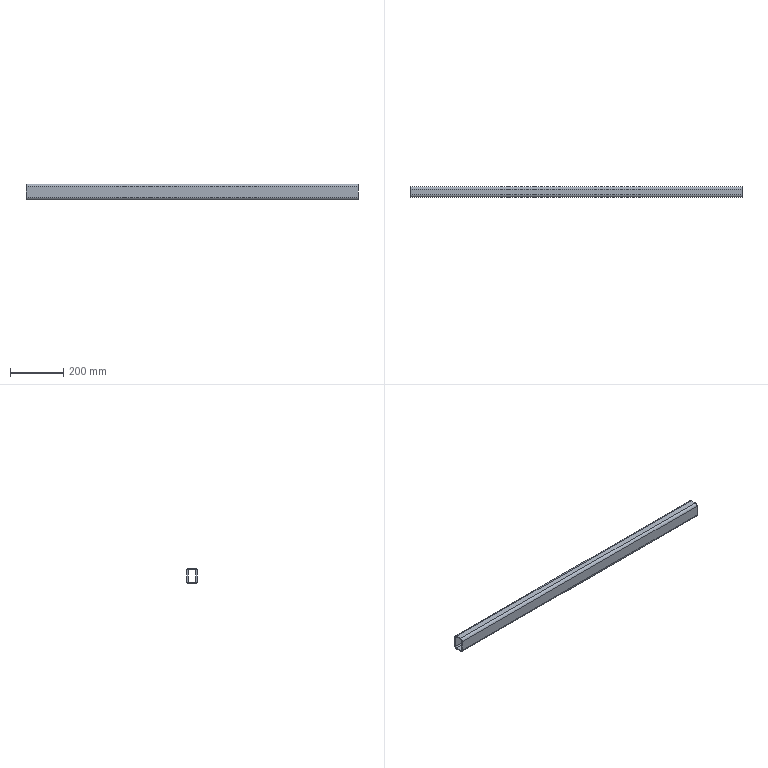Part | STEP file | HL4GD-1.30.108 base frame outer longitudinal beam--20251212 | 1 solid | 18 faces | box 1250 x 40 x 60 mm | volume 1044524 mm3 | plane 10 | cylinder 8 | commonest cylinder face diameters 10 x4 20 x4
STEP:
#1=CARTESIAN_POINT('',(0.,0.,0.));
#2=DIRECTION('',(0.,0.,1.));
#3=DIRECTION('',(1.,0.,0.));
#4=AXIS2_PLACEMENT_3D('',#1,#2,#3);
#5=CARTESIAN_POINT('',(1515.,1140.,410.));
#6=VERTEX_POINT('',#5);
#7=CARTESIAN_POINT('',(1515.,1145.,415.));
#8=VERTEX_POINT('',#7);
#9=CARTESIAN_POINT('',(1515.,1140.,415.));
#10=DIRECTION('',(1.,0.,0.));
#11=DIRECTION('',(0.,1.,0.));
#12=AXIS2_PLACEMENT_3D('',#9,#10,#11);
#13=CIRCLE('',#12,5.);
#14=CARTESIAN_POINT('',(2495.,1140.,415.));
#15=DIRECTION('',(1.,0.,0.));
#16=DIRECTION('',(0.,1.,0.));
#17=AXIS2_PLACEMENT_3D('',#14,#15,#16);
#18=CYLINDRICAL_SURFACE('',#17,5.);
#19=CARTESIAN_POINT('',(0.,-980.));
#20=DIRECTION('',(1.,0.));
#21=VECTOR('',#20,1.);
#22=LINE('',#19,#21);
#23=(GEOMETRIC_REPRESENTATION_CONTEXT(2)PARAMETRIC_REPRESENTATION_CONTEXT()REPRESENTATION_CONTEXT('',''));
#24=DEFINITIONAL_REPRESENTATION('',(#22),#23);
#25=PCURVE('',#18,#24);
#26=CARTESIAN_POINT('',(1515.,1326.07,281.07));
#27=DIRECTION('',(1.,0.,0.));
#28=DIRECTION('',(0.,1.,0.));
#29=AXIS2_PLACEMENT_3D('',#26,#27,#28);
#30=PLANE('',#29);
#31=CARTESIAN_POINT('',(-186.07,133.93));
#32=DIRECTION('',(1.,0.));
#33=AXIS2_PLACEMENT_2D('',#31,#32);
#34=CIRCLE('',#33,5.);
#35=(GEOMETRIC_REPRESENTATION_CONTEXT(2)PARAMETRIC_REPRESENTATION_CONTEXT()REPRESENTATION_CONTEXT('',''));
#36=DEFINITIONAL_REPRESENTATION('',(#34),#35);
#37=PCURVE('',#30,#36);
#38=SURFACE_CURVE('',#13,(#25,#37),.PCURVE_S1.);
#39=EDGE_CURVE('',#6,#8,#38,.T.);
#40=ORIENTED_EDGE('',*,*,#39,.T.);
#41=CARTESIAN_POINT('',(2765.,1145.,415.));
#42=VERTEX_POINT('',#41);
#43=CARTESIAN_POINT('',(2495.,1145.,415.));
#44=DIRECTION('',(1.,0.,0.));
#45=VECTOR('',#44,1.);
#46=LINE('',#43,#45);
#47=CARTESIAN_POINT('',(6.283,0.));
#48=DIRECTION('',(0.,1.));
#49=VECTOR('',#48,1.);
#50=LINE('',#47,#49);
#51=(GEOMETRIC_REPRESENTATION_CONTEXT(2)PARAMETRIC_REPRESENTATION_CONTEXT()REPRESENTATION_CONTEXT('',''));
#52=DEFINITIONAL_REPRESENTATION('',(#50),#51);
#53=PCURVE('',#18,#52);
#54=CARTESIAN_POINT('',(2495.,1145.,415.));
#55=DIRECTION('',(0.,-1.,0.));
#56=DIRECTION('',(0.,0.,-1.));
#57=AXIS2_PLACEMENT_3D('',#54,#55,#56);
#58=PLANE('',#57);
#59=CARTESIAN_POINT('',(0.,0.));
#60=DIRECTION('',(0.,1.));
#61=VECTOR('',#60,1.);
#62=LINE('',#59,#61);
#63=(GEOMETRIC_REPRESENTATION_CONTEXT(2)PARAMETRIC_REPRESENTATION_CONTEXT()REPRESENTATION_CONTEXT('',''));
#64=DEFINITIONAL_REPRESENTATION('',(#62),#63);
#65=PCURVE('',#58,#64);
#66=SURFACE_CURVE('',#46,(#53,#65),.PCURVE_S1.);
#67=EDGE_CURVE('',#8,#42,#66,.T.);
#68=ORIENTED_EDGE('',*,*,#67,.T.);
#69=CARTESIAN_POINT('',(2765.,1140.,410.));
#70=VERTEX_POINT('',#69);
#71=CARTESIAN_POINT('',(2765.,1140.,415.));
#72=DIRECTION('',(1.,0.,0.));
#73=DIRECTION('',(0.,0.,-1.));
#74=AXIS2_PLACEMENT_3D('',#71,#72,#73);
#75=CIRCLE('',#74,5.);
#76=CARTESIAN_POINT('',(4.712,270.));
#77=DIRECTION('',(1.,0.));
#78=VECTOR('',#77,1.);
#79=LINE('',#76,#78);
#80=(GEOMETRIC_REPRESENTATION_CONTEXT(2)PARAMETRIC_REPRESENTATION_CONTEXT()REPRESENTATION_CONTEXT('',''));
#81=DEFINITIONAL_REPRESENTATION('',(#79),#80);
#82=PCURVE('',#18,#81);
#83=CARTESIAN_POINT('',(2765.,910.,435.));
#84=DIRECTION('',(1.,0.,0.));
#85=DIRECTION('',(0.,0.,-1.));
#86=AXIS2_PLACEMENT_3D('',#83,#84,#85);
#87=PLANE('',#86);
#88=CARTESIAN_POINT('',(20.,230.));
#89=DIRECTION('',(1.,0.));
#90=AXIS2_PLACEMENT_2D('',#88,#89);
#91=CIRCLE('',#90,5.);
#92=(GEOMETRIC_REPRESENTATION_CONTEXT(2)PARAMETRIC_REPRESENTATION_CONTEXT()REPRESENTATION_CONTEXT('',''));
#93=DEFINITIONAL_REPRESENTATION('',(#91),#92);
#94=PCURVE('',#87,#93);
#95=SURFACE_CURVE('',#75,(#82,#94),.PCURVE_S1.);
#96=EDGE_CURVE('',#70,#42,#95,.T.);
#97=ORIENTED_EDGE('',*,*,#96,.F.);
#98=CARTESIAN_POINT('',(2495.,1140.,410.));
#99=DIRECTION('',(1.,0.,0.));
#100=VECTOR('',#99,1.);
#101=LINE('',#98,#100);
#102=CARTESIAN_POINT('',(4.712,0.));
#103=DIRECTION('',(0.,1.));
#104=VECTOR('',#103,1.);
#105=LINE('',#102,#104);
#106=(GEOMETRIC_REPRESENTATION_CONTEXT(2)PARAMETRIC_REPRESENTATION_CONTEXT()REPRESENTATION_CONTEXT('',''));
#107=DEFINITIONAL_REPRESENTATION('',(#105),#106);
#108=PCURVE('',#18,#107);
#109=CARTESIAN_POINT('',(2495.,1120.,410.));
#110=DIRECTION('',(0.,0.,1.));
#111=DIRECTION('',(0.,-1.,0.));
#112=AXIS2_PLACEMENT_3D('',#109,#110,#111);
#113=PLANE('',#112);
#114=CARTESIAN_POINT('',(-20.,0.));
#115=DIRECTION('',(0.,1.));
#116=VECTOR('',#115,1.);
#117=LINE('',#114,#116);
#118=(GEOMETRIC_REPRESENTATION_CONTEXT(2)PARAMETRIC_REPRESENTATION_CONTEXT()REPRESENTATION_CONTEXT('',''));
#119=DEFINITIONAL_REPRESENTATION('',(#117),#118);
#120=PCURVE('',#113,#119);
#121=SURFACE_CURVE('',#101,(#108,#120),.PCURVE_S1.);
#122=EDGE_CURVE('',#6,#70,#121,.T.);
#123=ORIENTED_EDGE('',*,*,#122,.F.);
#124=EDGE_LOOP('',(#40,#68,#97,#123));
#125=FACE_BOUND('',#124,.F.);
#126=ADVANCED_FACE('',(#125),#18,.F.);
#127=CARTESIAN_POINT('',(1515.,1120.,410.));
#128=VERTEX_POINT('',#127);
#129=CARTESIAN_POINT('',(2765.,1120.,410.));
#130=VERTEX_POINT('',#129);
#131=CARTESIAN_POINT('',(2495.,1120.,410.));
#132=DIRECTION('',(1.,0.,0.));
#133=VECTOR('',#132,1.);
#134=LINE('',#131,#133);
#135=CARTESIAN_POINT('',(0.,0.));
#136=DIRECTION('',(0.,1.));
#137=VECTOR('',#136,1.);
#138=LINE('',#135,#137);
#139=(GEOMETRIC_REPRESENTATION_CONTEXT(2)PARAMETRIC_REPRESENTATION_CONTEXT()REPRESENTATION_CONTEXT('',''));
#140=DEFINITIONAL_REPRESENTATION('',(#138),#139);
#141=PCURVE('',#113,#140);
#142=CARTESIAN_POINT('',(2495.,1120.,415.));
#143=DIRECTION('',(1.,0.,0.));
#144=DIRECTION('',(0.,1.,0.));
#145=AXIS2_PLACEMENT_3D('',#142,#143,#144);
#146=CYLINDRICAL_SURFACE('',#145,5.);
#147=CARTESIAN_POINT('',(4.712,0.));
#148=DIRECTION('',(0.,1.));
#149=VECTOR('',#148,1.);
#150=LINE('',#147,#149);
#151=(GEOMETRIC_REPRESENTATION_CONTEXT(2)PARAMETRIC_REPRESENTATION_CONTEXT()REPRESENTATION_CONTEXT('',''));
#152=DEFINITIONAL_REPRESENTATION('',(#150),#151);
#153=PCURVE('',#146,#152);
#154=SURFACE_CURVE('',#134,(#141,#153),.PCURVE_S1.);
#155=EDGE_CURVE('',#128,#130,#154,.T.);
#156=ORIENTED_EDGE('',*,*,#155,.T.);
#157=CARTESIAN_POINT('',(2765.,1120.,410.));
#158=DIRECTION('',(0.,1.,0.));
#159=VECTOR('',#158,1.);
#160=LINE('',#157,#159);
#161=CARTESIAN_POINT('',(0.,270.));
#162=DIRECTION('',(-1.,0.));
#163=VECTOR('',#162,1.);
#164=LINE('',#161,#163);
#165=(GEOMETRIC_REPRESENTATION_CONTEXT(2)PARAMETRIC_REPRESENTATION_CONTEXT()REPRESENTATION_CONTEXT('',''));
#166=DEFINITIONAL_REPRESENTATION('',(#164),#165);
#167=PCURVE('',#113,#166);
#168=CARTESIAN_POINT('',(25.,210.));
#169=DIRECTION('',(0.,1.));
#170=VECTOR('',#169,1.);
#171=LINE('',#168,#170);
#172=(GEOMETRIC_REPRESENTATION_CONTEXT(2)PARAMETRIC_REPRESENTATION_CONTEXT()REPRESENTATION_CONTEXT('',''));
#173=DEFINITIONAL_REPRESENTATION('',(#171),#172);
#174=PCURVE('',#87,#173);
#175=SURFACE_CURVE('',#160,(#167,#174),.PCURVE_S1.);
#176=EDGE_CURVE('',#130,#70,#175,.T.);
#177=ORIENTED_EDGE('',*,*,#176,.T.);
#178=ORIENTED_EDGE('',*,*,#122,.F.);
#179=CARTESIAN_POINT('',(1515.,1120.,410.));
#180=DIRECTION('',(0.,-1.,0.));
#181=VECTOR('',#180,1.);
#182=LINE('',#179,#181);
#183=CARTESIAN_POINT('',(0.,-980.));
#184=DIRECTION('',(1.,0.));
#185=VECTOR('',#184,1.);
#186=LINE('',#183,#185);
#187=(GEOMETRIC_REPRESENTATION_CONTEXT(2)PARAMETRIC_REPRESENTATION_CONTEXT()REPRESENTATION_CONTEXT('',''));
#188=DEFINITIONAL_REPRESENTATION('',(#186),#187);
#189=PCURVE('',#113,#188);
#190=CARTESIAN_POINT('',(-206.07,128.93));
#191=DIRECTION('',(-1.,0.));
#192=VECTOR('',#191,1.);
#193=LINE('',#190,#192);
#194=(GEOMETRIC_REPRESENTATION_CONTEXT(2)PARAMETRIC_REPRESENTATION_CONTEXT()REPRESENTATION_CONTEXT('',''));
#195=DEFINITIONAL_REPRESENTATION('',(#193),#194);
#196=PCURVE('',#30,#195);
#197=SURFACE_CURVE('',#182,(#189,#196),.PCURVE_S1.);
#198=EDGE_CURVE('',#6,#128,#197,.T.);
#199=ORIENTED_EDGE('',*,*,#198,.T.);
#200=EDGE_LOOP('',(#156,#177,#178,#199));
#201=FACE_BOUND('',#200,.T.);
#202=ADVANCED_FACE('',(#201),#113,.T.);
#203=CARTESIAN_POINT('',(1515.,1115.,415.));
#204=VERTEX_POINT('',#203);
#205=CARTESIAN_POINT('',(1515.,1120.,415.));
#206=DIRECTION('',(-1.,0.,0.));
#207=DIRECTION('',(0.,1.,0.));
#208=AXIS2_PLACEMENT_3D('',#205,#206,#207);
#209=CIRCLE('',#208,5.);
#210=CARTESIAN_POINT('',(6.283,-980.));
#211=DIRECTION('',(-1.,0.));
#212=VECTOR('',#211,1.);
#213=LINE('',#210,#212);
#214=(GEOMETRIC_REPRESENTATION_CONTEXT(2)PARAMETRIC_REPRESENTATION_CONTEXT()REPRESENTATION_CONTEXT('',''));
#215=DEFINITIONAL_REPRESENTATION('',(#213),#214);
#216=PCURVE('',#146,#215);
#217=CARTESIAN_POINT('',(-201.07,133.93));
#218=CARTESIAN_POINT('',(-201.07,125.27));
#219=CARTESIAN_POINT('',(-208.57,129.6));
#220=CARTESIAN_POINT('',(-216.07,133.93));
#221=CARTESIAN_POINT('',(-208.57,138.261));
#222=CARTESIAN_POINT('',(-201.07,142.591));
#223=CARTESIAN_POINT('',(-201.07,133.93));
#224=(BOUNDED_CURVE()B_SPLINE_CURVE(2,(#217,#218,#219,#220,#221,#222,#223),.UNSPECIFIED.,.T.,.F.)B_SPLINE_CURVE_WITH_KNOTS((1,2,2,2,2,1),(-2.094,0.,2.094,4.189,6.283,8.378),.UNSPECIFIED.)CURVE()GEOMETRIC_REPRESENTATION_ITEM()RATIONAL_B_SPLINE_CURVE((1.,0.5,1.,0.5,1.,0.5,1.))REPRESENTATION_ITEM(''));
#225=(GEOMETRIC_REPRESENTATION_CONTEXT(2)PARAMETRIC_REPRESENTATION_CONTEXT()REPRESENTATION_CONTEXT('',''));
#226=DEFINITIONAL_REPRESENTATION('',(#224),#225);
#227=PCURVE('',#30,#226);
#228=SURFACE_CURVE('',#209,(#216,#227),.PCURVE_S1.);
#229=EDGE_CURVE('',#128,#204,#228,.T.);
#230=ORIENTED_EDGE('',*,*,#229,.F.);
#231=ORIENTED_EDGE('',*,*,#155,.T.);
#232=CARTESIAN_POINT('',(2765.,1115.,415.));
#233=VERTEX_POINT('',#232);
#234=CARTESIAN_POINT('',(2765.,1120.,415.));
#235=DIRECTION('',(1.,0.,0.));
#236=DIRECTION('',(0.,0.,-1.));
#237=AXIS2_PLACEMENT_3D('',#234,#235,#236);
#238=CIRCLE('',#237,5.);
#239=CARTESIAN_POINT('',(-1.571,270.));
#240=DIRECTION('',(1.,0.));
#241=VECTOR('',#240,1.);
#242=LINE('',#239,#241);
#243=(GEOMETRIC_REPRESENTATION_CONTEXT(2)PARAMETRIC_REPRESENTATION_CONTEXT()REPRESENTATION_CONTEXT('',''));
#244=DEFINITIONAL_REPRESENTATION('',(#242),#243);
#245=PCURVE('',#146,#244);
#246=CARTESIAN_POINT('',(20.,210.));
#247=DIRECTION('',(1.,0.));
#248=AXIS2_PLACEMENT_2D('',#246,#247);
#249=CIRCLE('',#248,5.);
#250=(GEOMETRIC_REPRESENTATION_CONTEXT(2)PARAMETRIC_REPRESENTATION_CONTEXT()REPRESENTATION_CONTEXT('',''));
#251=DEFINITIONAL_REPRESENTATION('',(#249),#250);
#252=PCURVE('',#87,#251);
#253=SURFACE_CURVE('',#238,(#245,#252),.PCURVE_S1.);
#254=EDGE_CURVE('',#233,#130,#253,.T.);
#255=ORIENTED_EDGE('',*,*,#254,.F.);
#256=CARTESIAN_POINT('',(2495.,1115.,415.));
#257=DIRECTION('',(1.,0.,0.));
#258=VECTOR('',#257,1.);
#259=LINE('',#256,#258);
#260=CARTESIAN_POINT('',(3.142,0.));
#261=DIRECTION('',(0.,1.));
#262=VECTOR('',#261,1.);
#263=LINE('',#260,#262);
#264=(GEOMETRIC_REPRESENTATION_CONTEXT(2)PARAMETRIC_REPRESENTATION_CONTEXT()REPRESENTATION_CONTEXT('',''));
#265=DEFINITIONAL_REPRESENTATION('',(#263),#264);
#266=PCURVE('',#146,#265);
#267=CARTESIAN_POINT('',(2495.,1115.,455.));
#268=DIRECTION('',(0.,1.,0.));
#269=DIRECTION('',(0.,0.,1.));
#270=AXIS2_PLACEMENT_3D('',#267,#268,#269);
#271=PLANE('',#270);
#272=CARTESIAN_POINT('',(-40.,0.));
#273=DIRECTION('',(0.,1.));
#274=VECTOR('',#273,1.);
#275=LINE('',#272,#274);
#276=(GEOMETRIC_REPRESENTATION_CONTEXT(2)PARAMETRIC_REPRESENTATION_CONTEXT()REPRESENTATION_CONTEXT('',''));
#277=DEFINITIONAL_REPRESENTATION('',(#275),#276);
#278=PCURVE('',#271,#277);
#279=SURFACE_CURVE('',#259,(#266,#278),.PCURVE_S1.);
#280=EDGE_CURVE('',#204,#233,#279,.T.);
#281=ORIENTED_EDGE('',*,*,#280,.F.);
#282=EDGE_LOOP('',(#230,#231,#255,#281));
#283=FACE_BOUND('',#282,.F.);
#284=ADVANCED_FACE('',(#283),#146,.F.);
#285=CARTESIAN_POINT('',(1515.,1115.,455.));
#286=VERTEX_POINT('',#285);
#287=CARTESIAN_POINT('',(2765.,1115.,455.));
#288=VERTEX_POINT('',#287);
#289=CARTESIAN_POINT('',(2495.,1115.,455.));
#290=DIRECTION('',(1.,0.,0.));
#291=VECTOR('',#290,1.);
#292=LINE('',#289,#291);
#293=CARTESIAN_POINT('',(0.,0.));
#294=DIRECTION('',(0.,1.));
#295=VECTOR('',#294,1.);
#296=LINE('',#293,#295);
#297=(GEOMETRIC_REPRESENTATION_CONTEXT(2)PARAMETRIC_REPRESENTATION_CONTEXT()REPRESENTATION_CONTEXT('',''));
#298=DEFINITIONAL_REPRESENTATION('',(#296),#297);
#299=PCURVE('',#271,#298);
#300=CARTESIAN_POINT('',(2495.,1120.,455.));
#301=DIRECTION('',(1.,0.,0.));
#302=DIRECTION('',(0.,1.,0.));
#303=AXIS2_PLACEMENT_3D('',#300,#301,#302);
#304=CYLINDRICAL_SURFACE('',#303,5.);
#305=CARTESIAN_POINT('',(3.142,0.));
#306=DIRECTION('',(0.,1.));
#307=VECTOR('',#306,1.);
#308=LINE('',#305,#307);
#309=(GEOMETRIC_REPRESENTATION_CONTEXT(2)PARAMETRIC_REPRESENTATION_CONTEXT()REPRESENTATION_CONTEXT('',''));
#310=DEFINITIONAL_REPRESENTATION('',(#308),#309);
#311=PCURVE('',#304,#310);
#312=SURFACE_CURVE('',#292,(#299,#311),.PCURVE_S1.);
#313=EDGE_CURVE('',#286,#288,#312,.T.);
#314=ORIENTED_EDGE('',*,*,#313,.T.);
#315=CARTESIAN_POINT('',(2765.,1115.,455.));
#316=DIRECTION('',(0.,0.,-1.));
#317=VECTOR('',#316,1.);
#318=LINE('',#315,#317);
#319=CARTESIAN_POINT('',(0.,270.));
#320=DIRECTION('',(-1.,0.));
#321=VECTOR('',#320,1.);
#322=LINE('',#319,#321);
#323=(GEOMETRIC_REPRESENTATION_CONTEXT(2)PARAMETRIC_REPRESENTATION_CONTEXT()REPRESENTATION_CONTEXT('',''));
#324=DEFINITIONAL_REPRESENTATION('',(#322),#323);
#325=PCURVE('',#271,#324);
#326=CARTESIAN_POINT('',(-20.,205.));
#327=DIRECTION('',(1.,0.));
#328=VECTOR('',#327,1.);
#329=LINE('',#326,#328);
#330=(GEOMETRIC_REPRESENTATION_CONTEXT(2)PARAMETRIC_REPRESENTATION_CONTEXT()REPRESENTATION_CONTEXT('',''));
#331=DEFINITIONAL_REPRESENTATION('',(#329),#330);
#332=PCURVE('',#87,#331);
#333=SURFACE_CURVE('',#318,(#325,#332),.PCURVE_S1.);
#334=EDGE_CURVE('',#288,#233,#333,.T.);
#335=ORIENTED_EDGE('',*,*,#334,.T.);
#336=ORIENTED_EDGE('',*,*,#280,.F.);
#337=CARTESIAN_POINT('',(1515.,1115.,455.));
#338=DIRECTION('',(0.,0.,-1.));
#339=VECTOR('',#338,1.);
#340=LINE('',#337,#339);
#341=CARTESIAN_POINT('',(0.,-980.));
#342=DIRECTION('',(-1.,0.));
#343=VECTOR('',#342,1.);
#344=LINE('',#341,#343);
#345=(GEOMETRIC_REPRESENTATION_CONTEXT(2)PARAMETRIC_REPRESENTATION_CONTEXT()REPRESENTATION_CONTEXT('',''));
#346=DEFINITIONAL_REPRESENTATION('',(#344),#345);
#347=PCURVE('',#271,#346);
#348=CARTESIAN_POINT('',(-211.07,173.93));
#349=DIRECTION('',(0.,-1.));
#350=VECTOR('',#349,1.);
#351=LINE('',#348,#350);
#352=(GEOMETRIC_REPRESENTATION_CONTEXT(2)PARAMETRIC_REPRESENTATION_CONTEXT()REPRESENTATION_CONTEXT('',''));
#353=DEFINITIONAL_REPRESENTATION('',(#351),#352);
#354=PCURVE('',#30,#353);
#355=SURFACE_CURVE('',#340,(#347,#354),.PCURVE_S1.);
#356=EDGE_CURVE('',#286,#204,#355,.T.);
#357=ORIENTED_EDGE('',*,*,#356,.F.);
#358=EDGE_LOOP('',(#314,#335,#336,#357));
#359=FACE_BOUND('',#358,.T.);
#360=ADVANCED_FACE('',(#359),#271,.T.);
#361=CARTESIAN_POINT('',(1515.,1120.,460.));
#362=VERTEX_POINT('',#361);
#363=CARTESIAN_POINT('',(1515.,1120.,455.));
#364=DIRECTION('',(1.,0.,0.));
#365=DIRECTION('',(0.,1.,0.));
#366=AXIS2_PLACEMENT_3D('',#363,#364,#365);
#367=CIRCLE('',#366,5.);
#368=CARTESIAN_POINT('',(0.,-980.));
#369=DIRECTION('',(1.,0.));
#370=VECTOR('',#369,1.);
#371=LINE('',#368,#370);
#372=(GEOMETRIC_REPRESENTATION_CONTEXT(2)PARAMETRIC_REPRESENTATION_CONTEXT()REPRESENTATION_CONTEXT('',''));
#373=DEFINITIONAL_REPRESENTATION('',(#371),#372);
#374=PCURVE('',#304,#373);
#375=CARTESIAN_POINT('',(-206.07,173.93));
#376=DIRECTION('',(1.,0.));
#377=AXIS2_PLACEMENT_2D('',#375,#376);
#378=CIRCLE('',#377,5.);
#379=(GEOMETRIC_REPRESENTATION_CONTEXT(2)PARAMETRIC_REPRESENTATION_CONTEXT()REPRESENTATION_CONTEXT('',''));
#380=DEFINITIONAL_REPRESENTATION('',(#378),#379);
#381=PCURVE('',#30,#380);
#382=SURFACE_CURVE('',#367,(#374,#381),.PCURVE_S1.);
#383=EDGE_CURVE('',#362,#286,#382,.T.);
#384=ORIENTED_EDGE('',*,*,#383,.T.);
#385=ORIENTED_EDGE('',*,*,#313,.T.);
#386=CARTESIAN_POINT('',(2765.,1120.,460.));
#387=VERTEX_POINT('',#386);
#388=CARTESIAN_POINT('',(2765.,1120.,455.));
#389=DIRECTION('',(1.,0.,0.));
#390=DIRECTION('',(0.,0.,-1.));
#391=AXIS2_PLACEMENT_3D('',#388,#389,#390);
#392=CIRCLE('',#391,5.);
#393=CARTESIAN_POINT('',(-1.571,270.));
#394=DIRECTION('',(1.,0.));
#395=VECTOR('',#394,1.);
#396=LINE('',#393,#395);
#397=(GEOMETRIC_REPRESENTATION_CONTEXT(2)PARAMETRIC_REPRESENTATION_CONTEXT()REPRESENTATION_CONTEXT('',''));
#398=DEFINITIONAL_REPRESENTATION('',(#396),#397);
#399=PCURVE('',#304,#398);
#400=CARTESIAN_POINT('',(-20.,210.));
#401=DIRECTION('',(1.,0.));
#402=AXIS2_PLACEMENT_2D('',#400,#401);
#403=CIRCLE('',#402,5.);
#404=(GEOMETRIC_REPRESENTATION_CONTEXT(2)PARAMETRIC_REPRESENTATION_CONTEXT()REPRESENTATION_CONTEXT('',''));
#405=DEFINITIONAL_REPRESENTATION('',(#403),#404);
#406=PCURVE('',#87,#405);
#407=SURFACE_CURVE('',#392,(#399,#406),.PCURVE_S1.);
#408=EDGE_CURVE('',#387,#288,#407,.T.);
#409=ORIENTED_EDGE('',*,*,#408,.F.);
#410=CARTESIAN_POINT('',(2495.,1120.,460.));
#411=DIRECTION('',(1.,0.,0.));
#412=VECTOR('',#411,1.);
#413=LINE('',#410,#412);
#414=CARTESIAN_POINT('',(1.571,0.));
#415=DIRECTION('',(0.,1.));
#416=VECTOR('',#415,1.);
#417=LINE('',#414,#416);
#418=(GEOMETRIC_REPRESENTATION_CONTEXT(2)PARAMETRIC_REPRESENTATION_CONTEXT()REPRESENTATION_CONTEXT('',''));
#419=DEFINITIONAL_REPRESENTATION('',(#417),#418);
#420=PCURVE('',#304,#419);
#421=CARTESIAN_POINT('',(2495.,1140.,460.));
#422=DIRECTION('',(0.,0.,-1.));
#423=DIRECTION('',(0.,1.,0.));
#424=AXIS2_PLACEMENT_3D('',#421,#422,#423);
#425=PLANE('',#424);
#426=CARTESIAN_POINT('',(-20.,0.));
#427=DIRECTION('',(0.,1.));
#428=VECTOR('',#427,1.);
#429=LINE('',#426,#428);
#430=(GEOMETRIC_REPRESENTATION_CONTEXT(2)PARAMETRIC_REPRESENTATION_CONTEXT()REPRESENTATION_CONTEXT('',''));
#431=DEFINITIONAL_REPRESENTATION('',(#429),#430);
#432=PCURVE('',#425,#431);
#433=SURFACE_CURVE('',#413,(#420,#432),.PCURVE_S1.);
#434=EDGE_CURVE('',#362,#387,#433,.T.);
#435=ORIENTED_EDGE('',*,*,#434,.F.);
#436=EDGE_LOOP('',(#384,#385,#409,#435));
#437=FACE_BOUND('',#436,.F.);
#438=ADVANCED_FACE('',(#437),#304,.F.);
#439=CARTESIAN_POINT('',(1515.,1140.,460.));
#440=VERTEX_POINT('',#439);
#441=CARTESIAN_POINT('',(2765.,1140.,460.));
#442=VERTEX_POINT('',#441);
#443=CARTESIAN_POINT('',(2495.,1140.,460.));
#444=DIRECTION('',(1.,0.,0.));
#445=VECTOR('',#444,1.);
#446=LINE('',#443,#445);
#447=CARTESIAN_POINT('',(0.,0.));
#448=DIRECTION('',(0.,1.));
#449=VECTOR('',#448,1.);
#450=LINE('',#447,#449);
#451=(GEOMETRIC_REPRESENTATION_CONTEXT(2)PARAMETRIC_REPRESENTATION_CONTEXT()REPRESENTATION_CONTEXT('',''));
#452=DEFINITIONAL_REPRESENTATION('',(#450),#451);
#453=PCURVE('',#425,#452);
#454=CARTESIAN_POINT('',(2495.,1140.,455.));
#455=DIRECTION('',(1.,0.,0.));
#456=DIRECTION('',(0.,1.,0.));
#457=AXIS2_PLACEMENT_3D('',#454,#455,#456);
#458=CYLINDRICAL_SURFACE('',#457,5.);
#459=CARTESIAN_POINT('',(1.571,0.));
#460=DIRECTION('',(0.,1.));
#461=VECTOR('',#460,1.);
#462=LINE('',#459,#461);
#463=(GEOMETRIC_REPRESENTATION_CONTEXT(2)PARAMETRIC_REPRESENTATION_CONTEXT()REPRESENTATION_CONTEXT('',''));
#464=DEFINITIONAL_REPRESENTATION('',(#462),#463);
#465=PCURVE('',#458,#464);
#466=SURFACE_CURVE('',#446,(#453,#465),.PCURVE_S1.);
#467=EDGE_CURVE('',#440,#442,#466,.T.);
#468=ORIENTED_EDGE('',*,*,#467,.T.);
#469=CARTESIAN_POINT('',(2765.,1140.,460.));
#470=DIRECTION('',(0.,-1.,0.));
#471=VECTOR('',#470,1.);
#472=LINE('',#469,#471);
#473=CARTESIAN_POINT('',(0.,270.));
#474=DIRECTION('',(-1.,0.));
#475=VECTOR('',#474,1.);
#476=LINE('',#473,#475);
#477=(GEOMETRIC_REPRESENTATION_CONTEXT(2)PARAMETRIC_REPRESENTATION_CONTEXT()REPRESENTATION_CONTEXT('',''));
#478=DEFINITIONAL_REPRESENTATION('',(#476),#477);
#479=PCURVE('',#425,#478);
#480=CARTESIAN_POINT('',(-25.,230.));
#481=DIRECTION('',(0.,-1.));
#482=VECTOR('',#481,1.);
#483=LINE('',#480,#482);
#484=(GEOMETRIC_REPRESENTATION_CONTEXT(2)PARAMETRIC_REPRESENTATION_CONTEXT()REPRESENTATION_CONTEXT('',''));
#485=DEFINITIONAL_REPRESENTATION('',(#483),#484);
#486=PCURVE('',#87,#485);
#487=SURFACE_CURVE('',#472,(#479,#486),.PCURVE_S1.);
#488=EDGE_CURVE('',#442,#387,#487,.T.);
#489=ORIENTED_EDGE('',*,*,#488,.T.);
#490=ORIENTED_EDGE('',*,*,#434,.F.);
#491=CARTESIAN_POINT('',(1515.,1140.,460.));
#492=DIRECTION('',(0.,-1.,0.));
#493=VECTOR('',#492,1.);
#494=LINE('',#491,#493);
#495=CARTESIAN_POINT('',(0.,-980.));
#496=DIRECTION('',(-1.,0.));
#497=VECTOR('',#496,1.);
#498=LINE('',#495,#497);
#499=(GEOMETRIC_REPRESENTATION_CONTEXT(2)PARAMETRIC_REPRESENTATION_CONTEXT()REPRESENTATION_CONTEXT('',''));
#500=DEFINITIONAL_REPRESENTATION('',(#498),#499);
#501=PCURVE('',#425,#500);
#502=CARTESIAN_POINT('',(-186.07,178.93));
#503=DIRECTION('',(-1.,0.));
#504=VECTOR('',#503,1.);
#505=LINE('',#502,#504);
#506=(GEOMETRIC_REPRESENTATION_CONTEXT(2)PARAMETRIC_REPRESENTATION_CONTEXT()REPRESENTATION_CONTEXT('',''));
#507=DEFINITIONAL_REPRESENTATION('',(#505),#506);
#508=PCURVE('',#30,#507);
#509=SURFACE_CURVE('',#494,(#501,#508),.PCURVE_S1.);
#510=EDGE_CURVE('',#440,#362,#509,.T.);
#511=ORIENTED_EDGE('',*,*,#510,.F.);
#512=EDGE_LOOP('',(#468,#489,#490,#511));
#513=FACE_BOUND('',#512,.T.);
#514=ADVANCED_FACE('',(#513),#425,.T.);
#515=CARTESIAN_POINT('',(1515.,1145.,455.));
#516=VERTEX_POINT('',#515);
#517=CARTESIAN_POINT('',(1515.,1140.,455.));
#518=DIRECTION('',(-1.,0.,0.));
#519=DIRECTION('',(0.,1.,0.));
#520=AXIS2_PLACEMENT_3D('',#517,#518,#519);
#521=CIRCLE('',#520,5.);
#522=CARTESIAN_POINT('',(6.283,-980.));
#523=DIRECTION('',(-1.,0.));
#524=VECTOR('',#523,1.);
#525=LINE('',#522,#524);
#526=(GEOMETRIC_REPRESENTATION_CONTEXT(2)PARAMETRIC_REPRESENTATION_CONTEXT()REPRESENTATION_CONTEXT('',''));
#527=DEFINITIONAL_REPRESENTATION('',(#525),#526);
#528=PCURVE('',#458,#527);
#529=CARTESIAN_POINT('',(-181.07,173.93));
#530=CARTESIAN_POINT('',(-181.07,165.27));
#531=CARTESIAN_POINT('',(-188.57,169.6));
#532=CARTESIAN_POINT('',(-196.07,173.93));
#533=CARTESIAN_POINT('',(-188.57,178.261));
#534=CARTESIAN_POINT('',(-181.07,182.591));
#535=CARTESIAN_POINT('',(-181.07,173.93));
#536=(BOUNDED_CURVE()B_SPLINE_CURVE(2,(#529,#530,#531,#532,#533,#534,#535),.UNSPECIFIED.,.T.,.F.)B_SPLINE_CURVE_WITH_KNOTS((1,2,2,2,2,1),(-2.094,0.,2.094,4.189,6.283,8.378),.UNSPECIFIED.)CURVE()GEOMETRIC_REPRESENTATION_ITEM()RATIONAL_B_SPLINE_CURVE((1.,0.5,1.,0.5,1.,0.5,1.))REPRESENTATION_ITEM(''));
#537=(GEOMETRIC_REPRESENTATION_CONTEXT(2)PARAMETRIC_REPRESENTATION_CONTEXT()REPRESENTATION_CONTEXT('',''));
#538=DEFINITIONAL_REPRESENTATION('',(#536),#537);
#539=PCURVE('',#30,#538);
#540=SURFACE_CURVE('',#521,(#528,#539),.PCURVE_S1.);
#541=EDGE_CURVE('',#440,#516,#540,.T.);
#542=ORIENTED_EDGE('',*,*,#541,.F.);
#543=ORIENTED_EDGE('',*,*,#467,.T.);
#544=CARTESIAN_POINT('',(2765.,1145.,455.));
#545=VERTEX_POINT('',#544);
#546=CARTESIAN_POINT('',(2765.,1140.,455.));
#547=DIRECTION('',(1.,0.,0.));
#548=DIRECTION('',(0.,0.,-1.));
#549=AXIS2_PLACEMENT_3D('',#546,#547,#548);
#550=CIRCLE('',#549,5.);
#551=CARTESIAN_POINT('',(-1.571,270.));
#552=DIRECTION('',(1.,0.));
#553=VECTOR('',#552,1.);
#554=LINE('',#551,#553);
#555=(GEOMETRIC_REPRESENTATION_CONTEXT(2)PARAMETRIC_REPRESENTATION_CONTEXT()REPRESENTATION_CONTEXT('',''));
#556=DEFINITIONAL_REPRESENTATION('',(#554),#555);
#557=PCURVE('',#458,#556);
#558=CARTESIAN_POINT('',(-20.,230.));
#559=DIRECTION('',(1.,0.));
#560=AXIS2_PLACEMENT_2D('',#558,#559);
#561=CIRCLE('',#560,5.);
#562=(GEOMETRIC_REPRESENTATION_CONTEXT(2)PARAMETRIC_REPRESENTATION_CONTEXT()REPRESENTATION_CONTEXT('',''));
#563=DEFINITIONAL_REPRESENTATION('',(#561),#562);
#564=PCURVE('',#87,#563);
#565=SURFACE_CURVE('',#550,(#557,#564),.PCURVE_S1.);
#566=EDGE_CURVE('',#545,#442,#565,.T.);
#567=ORIENTED_EDGE('',*,*,#566,.F.);
#568=CARTESIAN_POINT('',(2495.,1145.,455.));
#569=DIRECTION('',(1.,0.,0.));
#570=VECTOR('',#569,1.);
#571=LINE('',#568,#570);
#572=CARTESIAN_POINT('',(0.,0.));
#573=DIRECTION('',(0.,1.));
#574=VECTOR('',#573,1.);
#575=LINE('',#572,#574);
#576=(GEOMETRIC_REPRESENTATION_CONTEXT(2)PARAMETRIC_REPRESENTATION_CONTEXT()REPRESENTATION_CONTEXT('',''));
#577=DEFINITIONAL_REPRESENTATION('',(#575),#576);
#578=PCURVE('',#458,#577);
#579=CARTESIAN_POINT('',(-40.,0.));
#580=DIRECTION('',(0.,1.));
#581=VECTOR('',#580,1.);
#582=LINE('',#579,#581);
#583=(GEOMETRIC_REPRESENTATION_CONTEXT(2)PARAMETRIC_REPRESENTATION_CONTEXT()REPRESENTATION_CONTEXT('',''));
#584=DEFINITIONAL_REPRESENTATION('',(#582),#583);
#585=PCURVE('',#58,#584);
#586=SURFACE_CURVE('',#571,(#578,#585),.PCURVE_S1.);
#587=EDGE_CURVE('',#516,#545,#586,.T.);
#588=ORIENTED_EDGE('',*,*,#587,.F.);
#589=EDGE_LOOP('',(#542,#543,#567,#588));
#590=FACE_BOUND('',#589,.F.);
#591=ADVANCED_FACE('',(#590),#458,.F.);
#592=CARTESIAN_POINT('',(1515.,1110.,415.));
#593=VERTEX_POINT('',#592);
#594=CARTESIAN_POINT('',(2765.,1110.,415.));
#595=VERTEX_POINT('',#594);
#596=CARTESIAN_POINT('',(2495.,1110.,415.));
#597=DIRECTION('',(1.,0.,0.));
#598=VECTOR('',#597,1.);
#599=LINE('',#596,#598);
#600=CARTESIAN_POINT('',(2495.,1110.,455.));
#601=DIRECTION('',(0.,1.,0.));
#602=DIRECTION('',(0.,0.,1.));
#603=AXIS2_PLACEMENT_3D('',#600,#601,#602);
#604=PLANE('',#603);
#605=CARTESIAN_POINT('',(-40.,0.));
#606=DIRECTION('',(0.,1.));
#607=VECTOR('',#606,1.);
#608=LINE('',#605,#607);
#609=(GEOMETRIC_REPRESENTATION_CONTEXT(2)PARAMETRIC_REPRESENTATION_CONTEXT()REPRESENTATION_CONTEXT('',''));
#610=DEFINITIONAL_REPRESENTATION('',(#608),#609);
#611=PCURVE('',#604,#610);
#612=CARTESIAN_POINT('',(2495.,1120.,415.));
#613=DIRECTION('',(1.,0.,0.));
#614=DIRECTION('',(0.,1.,0.));
#615=AXIS2_PLACEMENT_3D('',#612,#613,#614);
#616=CYLINDRICAL_SURFACE('',#615,10.);
#617=CARTESIAN_POINT('',(3.142,0.));
#618=DIRECTION('',(0.,1.));
#619=VECTOR('',#618,1.);
#620=LINE('',#617,#619);
#621=(GEOMETRIC_REPRESENTATION_CONTEXT(2)PARAMETRIC_REPRESENTATION_CONTEXT()REPRESENTATION_CONTEXT('',''));
#622=DEFINITIONAL_REPRESENTATION('',(#620),#621);
#623=PCURVE('',#616,#622);
#624=SURFACE_CURVE('',#599,(#611,#623),.PCURVE_S1.);
#625=EDGE_CURVE('',#593,#595,#624,.T.);
#626=ORIENTED_EDGE('',*,*,#625,.T.);
#627=CARTESIAN_POINT('',(2765.,1110.,455.));
#628=VERTEX_POINT('',#627);
#629=CARTESIAN_POINT('',(2765.,1110.,455.));
#630=DIRECTION('',(0.,0.,1.));
#631=VECTOR('',#630,1.);
#632=LINE('',#629,#631);
#633=CARTESIAN_POINT('',(0.,270.));
#634=DIRECTION('',(1.,0.));
#635=VECTOR('',#634,1.);
#636=LINE('',#633,#635);
#637=(GEOMETRIC_REPRESENTATION_CONTEXT(2)PARAMETRIC_REPRESENTATION_CONTEXT()REPRESENTATION_CONTEXT('',''));
#638=DEFINITIONAL_REPRESENTATION('',(#636),#637);
#639=PCURVE('',#604,#638);
#640=CARTESIAN_POINT('',(-20.,200.));
#641=DIRECTION('',(-1.,0.));
#642=VECTOR('',#641,1.);
#643=LINE('',#640,#642);
#644=(GEOMETRIC_REPRESENTATION_CONTEXT(2)PARAMETRIC_REPRESENTATION_CONTEXT()REPRESENTATION_CONTEXT('',''));
#645=DEFINITIONAL_REPRESENTATION('',(#643),#644);
#646=PCURVE('',#87,#645);
#647=SURFACE_CURVE('',#632,(#639,#646),.PCURVE_S1.);
#648=EDGE_CURVE('',#595,#628,#647,.T.);
#649=ORIENTED_EDGE('',*,*,#648,.T.);
#650=CARTESIAN_POINT('',(1515.,1110.,455.));
#651=VERTEX_POINT('',#650);
#652=CARTESIAN_POINT('',(2495.,1110.,455.));
#653=DIRECTION('',(1.,0.,0.));
#654=VECTOR('',#653,1.);
#655=LINE('',#652,#654);
#656=CARTESIAN_POINT('',(0.,0.));
#657=DIRECTION('',(0.,1.));
#658=VECTOR('',#657,1.);
#659=LINE('',#656,#658);
#660=(GEOMETRIC_REPRESENTATION_CONTEXT(2)PARAMETRIC_REPRESENTATION_CONTEXT()REPRESENTATION_CONTEXT('',''));
#661=DEFINITIONAL_REPRESENTATION('',(#659),#660);
#662=PCURVE('',#604,#661);
#663=CARTESIAN_POINT('',(2495.,1120.,455.));
#664=DIRECTION('',(1.,0.,0.));
#665=DIRECTION('',(0.,1.,0.));
#666=AXIS2_PLACEMENT_3D('',#663,#664,#665);
#667=CYLINDRICAL_SURFACE('',#666,10.);
#668=CARTESIAN_POINT('',(3.142,0.));
#669=DIRECTION('',(0.,1.));
#670=VECTOR('',#669,1.);
#671=LINE('',#668,#670);
#672=(GEOMETRIC_REPRESENTATION_CONTEXT(2)PARAMETRIC_REPRESENTATION_CONTEXT()REPRESENTATION_CONTEXT('',''));
#673=DEFINITIONAL_REPRESENTATION('',(#671),#672);
#674=PCURVE('',#667,#673);
#675=SURFACE_CURVE('',#655,(#662,#674),.PCURVE_S1.);
#676=EDGE_CURVE('',#651,#628,#675,.T.);
#677=ORIENTED_EDGE('',*,*,#676,.F.);
#678=CARTESIAN_POINT('',(1515.,1110.,455.));
#679=DIRECTION('',(0.,0.,1.));
#680=VECTOR('',#679,1.);
#681=LINE('',#678,#680);
#682=CARTESIAN_POINT('',(0.,-980.));
#683=DIRECTION('',(1.,0.));
#684=VECTOR('',#683,1.);
#685=LINE('',#682,#684);
#686=(GEOMETRIC_REPRESENTATION_CONTEXT(2)PARAMETRIC_REPRESENTATION_CONTEXT()REPRESENTATION_CONTEXT('',''));
#687=DEFINITIONAL_REPRESENTATION('',(#685),#686);
#688=PCURVE('',#604,#687);
#689=CARTESIAN_POINT('',(-216.07,173.93));
#690=DIRECTION('',(0.,1.));
#691=VECTOR('',#690,1.);
#692=LINE('',#689,#691);
#693=(GEOMETRIC_REPRESENTATION_CONTEXT(2)PARAMETRIC_REPRESENTATION_CONTEXT()REPRESENTATION_CONTEXT('',''));
#694=DEFINITIONAL_REPRESENTATION('',(#692),#693);
#695=PCURVE('',#30,#694);
#696=SURFACE_CURVE('',#681,(#688,#695),.PCURVE_S1.);
#697=EDGE_CURVE('',#593,#651,#696,.T.);
#698=ORIENTED_EDGE('',*,*,#697,.F.);
#699=EDGE_LOOP('',(#626,#649,#677,#698));
#700=FACE_BOUND('',#699,.T.);
#701=ADVANCED_FACE('',(#700),#604,.F.);
#702=CARTESIAN_POINT('',(1515.,1120.,405.));
#703=VERTEX_POINT('',#702);
#704=CARTESIAN_POINT('',(2765.,1120.,405.));
#705=VERTEX_POINT('',#704);
#706=CARTESIAN_POINT('',(2495.,1120.,405.));
#707=DIRECTION('',(1.,0.,0.));
#708=VECTOR('',#707,1.);
#709=LINE('',#706,#708);
#710=CARTESIAN_POINT('',(4.712,0.));
#711=DIRECTION('',(0.,1.));
#712=VECTOR('',#711,1.);
#713=LINE('',#710,#712);
#714=(GEOMETRIC_REPRESENTATION_CONTEXT(2)PARAMETRIC_REPRESENTATION_CONTEXT()REPRESENTATION_CONTEXT('',''));
#715=DEFINITIONAL_REPRESENTATION('',(#713),#714);
#716=PCURVE('',#616,#715);
#717=CARTESIAN_POINT('',(2495.,1120.,405.));
#718=DIRECTION('',(0.,0.,1.));
#719=DIRECTION('',(0.,-1.,0.));
#720=AXIS2_PLACEMENT_3D('',#717,#718,#719);
#721=PLANE('',#720);
#722=CARTESIAN_POINT('',(0.,0.));
#723=DIRECTION('',(0.,1.));
#724=VECTOR('',#723,1.);
#725=LINE('',#722,#724);
#726=(GEOMETRIC_REPRESENTATION_CONTEXT(2)PARAMETRIC_REPRESENTATION_CONTEXT()REPRESENTATION_CONTEXT('',''));
#727=DEFINITIONAL_REPRESENTATION('',(#725),#726);
#728=PCURVE('',#721,#727);
#729=SURFACE_CURVE('',#709,(#716,#728),.PCURVE_S1.);
#730=EDGE_CURVE('',#703,#705,#729,.T.);
#731=ORIENTED_EDGE('',*,*,#730,.T.);
#732=CARTESIAN_POINT('',(2765.,1120.,415.));
#733=DIRECTION('',(-1.,0.,0.));
#734=DIRECTION('',(0.,0.,-1.));
#735=AXIS2_PLACEMENT_3D('',#732,#733,#734);
#736=CIRCLE('',#735,10.);
#737=CARTESIAN_POINT('',(4.712,270.));
#738=DIRECTION('',(-1.,0.));
#739=VECTOR('',#738,1.);
#740=LINE('',#737,#739);
#741=(GEOMETRIC_REPRESENTATION_CONTEXT(2)PARAMETRIC_REPRESENTATION_CONTEXT()REPRESENTATION_CONTEXT('',''));
#742=DEFINITIONAL_REPRESENTATION('',(#740),#741);
#743=PCURVE('',#616,#742);
#744=CARTESIAN_POINT('',(30.,210.));
#745=CARTESIAN_POINT('',(30.,192.679));
#746=CARTESIAN_POINT('',(15.,201.34));
#747=CARTESIAN_POINT('',(0.,210.));
#748=CARTESIAN_POINT('',(15.,218.66));
#749=CARTESIAN_POINT('',(30.,227.321));
#750=CARTESIAN_POINT('',(30.,210.));
#751=(BOUNDED_CURVE()B_SPLINE_CURVE(2,(#744,#745,#746,#747,#748,#749,#750),.UNSPECIFIED.,.T.,.F.)B_SPLINE_CURVE_WITH_KNOTS((1,2,2,2,2,1),(-2.094,0.,2.094,4.189,6.283,8.378),.UNSPECIFIED.)CURVE()GEOMETRIC_REPRESENTATION_ITEM()RATIONAL_B_SPLINE_CURVE((1.,0.5,1.,0.5,1.,0.5,1.))REPRESENTATION_ITEM(''));
#752=(GEOMETRIC_REPRESENTATION_CONTEXT(2)PARAMETRIC_REPRESENTATION_CONTEXT()REPRESENTATION_CONTEXT('',''));
#753=DEFINITIONAL_REPRESENTATION('',(#751),#752);
#754=PCURVE('',#87,#753);
#755=SURFACE_CURVE('',#736,(#743,#754),.PCURVE_S1.);
#756=EDGE_CURVE('',#705,#595,#755,.T.);
#757=ORIENTED_EDGE('',*,*,#756,.T.);
#758=ORIENTED_EDGE('',*,*,#625,.F.);
#759=CARTESIAN_POINT('',(1515.,1120.,415.));
#760=DIRECTION('',(-1.,0.,0.));
#761=DIRECTION('',(0.,1.,0.));
#762=AXIS2_PLACEMENT_3D('',#759,#760,#761);
#763=CIRCLE('',#762,10.);
#764=CARTESIAN_POINT('',(6.283,-980.));
#765=DIRECTION('',(-1.,0.));
#766=VECTOR('',#765,1.);
#767=LINE('',#764,#766);
#768=(GEOMETRIC_REPRESENTATION_CONTEXT(2)PARAMETRIC_REPRESENTATION_CONTEXT()REPRESENTATION_CONTEXT('',''));
#769=DEFINITIONAL_REPRESENTATION('',(#767),#768);
#770=PCURVE('',#616,#769);
#771=CARTESIAN_POINT('',(-196.07,133.93));
#772=CARTESIAN_POINT('',(-196.07,116.61));
#773=CARTESIAN_POINT('',(-211.07,125.27));
#774=CARTESIAN_POINT('',(-226.07,133.93));
#775=CARTESIAN_POINT('',(-211.07,142.591));
#776=CARTESIAN_POINT('',(-196.07,151.251));
#777=CARTESIAN_POINT('',(-196.07,133.93));
#778=(BOUNDED_CURVE()B_SPLINE_CURVE(2,(#771,#772,#773,#774,#775,#776,#777),.UNSPECIFIED.,.T.,.F.)B_SPLINE_CURVE_WITH_KNOTS((1,2,2,2,2,1),(-2.094,0.,2.094,4.189,6.283,8.378),.UNSPECIFIED.)CURVE()GEOMETRIC_REPRESENTATION_ITEM()RATIONAL_B_SPLINE_CURVE((1.,0.5,1.,0.5,1.,0.5,1.))REPRESENTATION_ITEM(''));
#779=(GEOMETRIC_REPRESENTATION_CONTEXT(2)PARAMETRIC_REPRESENTATION_CONTEXT()REPRESENTATION_CONTEXT('',''));
#780=DEFINITIONAL_REPRESENTATION('',(#778),#779);
#781=PCURVE('',#30,#780);
#782=SURFACE_CURVE('',#763,(#770,#781),.PCURVE_S1.);
#783=EDGE_CURVE('',#703,#593,#782,.T.);
#784=ORIENTED_EDGE('',*,*,#783,.F.);
#785=EDGE_LOOP('',(#731,#757,#758,#784));
#786=FACE_BOUND('',#785,.T.);
#787=ADVANCED_FACE('',(#786),#616,.T.);
#788=CARTESIAN_POINT('',(1515.,1140.,405.));
#789=VERTEX_POINT('',#788);
#790=CARTESIAN_POINT('',(2765.,1140.,405.));
#791=VERTEX_POINT('',#790);
#792=CARTESIAN_POINT('',(2495.,1140.,405.));
#793=DIRECTION('',(1.,0.,0.));
#794=VECTOR('',#793,1.);
#795=LINE('',#792,#794);
#796=CARTESIAN_POINT('',(-20.,0.));
#797=DIRECTION('',(0.,1.));
#798=VECTOR('',#797,1.);
#799=LINE('',#796,#798);
#800=(GEOMETRIC_REPRESENTATION_CONTEXT(2)PARAMETRIC_REPRESENTATION_CONTEXT()REPRESENTATION_CONTEXT('',''));
#801=DEFINITIONAL_REPRESENTATION('',(#799),#800);
#802=PCURVE('',#721,#801);
#803=CARTESIAN_POINT('',(2495.,1140.,415.));
#804=DIRECTION('',(1.,0.,0.));
#805=DIRECTION('',(0.,1.,0.));
#806=AXIS2_PLACEMENT_3D('',#803,#804,#805);
#807=CYLINDRICAL_SURFACE('',#806,10.);
#808=CARTESIAN_POINT('',(4.712,0.));
#809=DIRECTION('',(0.,1.));
#810=VECTOR('',#809,1.);
#811=LINE('',#808,#810);
#812=(GEOMETRIC_REPRESENTATION_CONTEXT(2)PARAMETRIC_REPRESENTATION_CONTEXT()REPRESENTATION_CONTEXT('',''));
#813=DEFINITIONAL_REPRESENTATION('',(#811),#812);
#814=PCURVE('',#807,#813);
#815=SURFACE_CURVE('',#795,(#802,#814),.PCURVE_S1.);
#816=EDGE_CURVE('',#789,#791,#815,.T.);
#817=ORIENTED_EDGE('',*,*,#816,.T.);
#818=CARTESIAN_POINT('',(2765.,1120.,405.));
#819=DIRECTION('',(0.,-1.,0.));
#820=VECTOR('',#819,1.);
#821=LINE('',#818,#820);
#822=CARTESIAN_POINT('',(0.,270.));
#823=DIRECTION('',(1.,0.));
#824=VECTOR('',#823,1.);
#825=LINE('',#822,#824);
#826=(GEOMETRIC_REPRESENTATION_CONTEXT(2)PARAMETRIC_REPRESENTATION_CONTEXT()REPRESENTATION_CONTEXT('',''));
#827=DEFINITIONAL_REPRESENTATION('',(#825),#826);
#828=PCURVE('',#721,#827);
#829=CARTESIAN_POINT('',(30.,210.));
#830=DIRECTION('',(0.,-1.));
#831=VECTOR('',#830,1.);
#832=LINE('',#829,#831);
#833=(GEOMETRIC_REPRESENTATION_CONTEXT(2)PARAMETRIC_REPRESENTATION_CONTEXT()REPRESENTATION_CONTEXT('',''));
#834=DEFINITIONAL_REPRESENTATION('',(#832),#833);
#835=PCURVE('',#87,#834);
#836=SURFACE_CURVE('',#821,(#828,#835),.PCURVE_S1.);
#837=EDGE_CURVE('',#791,#705,#836,.T.);
#838=ORIENTED_EDGE('',*,*,#837,.T.);
#839=ORIENTED_EDGE('',*,*,#730,.F.);
#840=CARTESIAN_POINT('',(1515.,1120.,405.));
#841=DIRECTION('',(0.,-1.,0.));
#842=VECTOR('',#841,1.);
#843=LINE('',#840,#842);
#844=CARTESIAN_POINT('',(0.,-980.));
#845=DIRECTION('',(1.,0.));
#846=VECTOR('',#845,1.);
#847=LINE('',#844,#846);
#848=(GEOMETRIC_REPRESENTATION_CONTEXT(2)PARAMETRIC_REPRESENTATION_CONTEXT()REPRESENTATION_CONTEXT('',''));
#849=DEFINITIONAL_REPRESENTATION('',(#847),#848);
#850=PCURVE('',#721,#849);
#851=CARTESIAN_POINT('',(-206.07,123.93));
#852=DIRECTION('',(-1.,0.));
#853=VECTOR('',#852,1.);
#854=LINE('',#851,#853);
#855=(GEOMETRIC_REPRESENTATION_CONTEXT(2)PARAMETRIC_REPRESENTATION_CONTEXT()REPRESENTATION_CONTEXT('',''));
#856=DEFINITIONAL_REPRESENTATION('',(#854),#855);
#857=PCURVE('',#30,#856);
#858=SURFACE_CURVE('',#843,(#850,#857),.PCURVE_S1.);
#859=EDGE_CURVE('',#789,#703,#858,.T.);
#860=ORIENTED_EDGE('',*,*,#859,.F.);
#861=EDGE_LOOP('',(#817,#838,#839,#860));
#862=FACE_BOUND('',#861,.T.);
#863=ADVANCED_FACE('',(#862),#721,.F.);
#864=CARTESIAN_POINT('',(1515.,1150.,415.));
#865=VERTEX_POINT('',#864);
#866=CARTESIAN_POINT('',(2765.,1150.,415.));
#867=VERTEX_POINT('',#866);
#868=CARTESIAN_POINT('',(2495.,1150.,415.));
#869=DIRECTION('',(1.,0.,0.));
#870=VECTOR('',#869,1.);
#871=LINE('',#868,#870);
#872=CARTESIAN_POINT('',(6.283,0.));
#873=DIRECTION('',(0.,1.));
#874=VECTOR('',#873,1.);
#875=LINE('',#872,#874);
#876=(GEOMETRIC_REPRESENTATION_CONTEXT(2)PARAMETRIC_REPRESENTATION_CONTEXT()REPRESENTATION_CONTEXT('',''));
#877=DEFINITIONAL_REPRESENTATION('',(#875),#876);
#878=PCURVE('',#807,#877);
#879=CARTESIAN_POINT('',(2495.,1150.,415.));
#880=DIRECTION('',(0.,-1.,0.));
#881=DIRECTION('',(0.,0.,-1.));
#882=AXIS2_PLACEMENT_3D('',#879,#880,#881);
#883=PLANE('',#882);
#884=CARTESIAN_POINT('',(0.,0.));
#885=DIRECTION('',(0.,1.));
#886=VECTOR('',#885,1.);
#887=LINE('',#884,#886);
#888=(GEOMETRIC_REPRESENTATION_CONTEXT(2)PARAMETRIC_REPRESENTATION_CONTEXT()REPRESENTATION_CONTEXT('',''));
#889=DEFINITIONAL_REPRESENTATION('',(#887),#888);
#890=PCURVE('',#883,#889);
#891=SURFACE_CURVE('',#871,(#878,#890),.PCURVE_S1.);
#892=EDGE_CURVE('',#865,#867,#891,.T.);
#893=ORIENTED_EDGE('',*,*,#892,.T.);
#894=CARTESIAN_POINT('',(2765.,1140.,415.));
#895=DIRECTION('',(-1.,0.,0.));
#896=DIRECTION('',(0.,0.,-1.));
#897=AXIS2_PLACEMENT_3D('',#894,#895,#896);
#898=CIRCLE('',#897,10.);
#899=CARTESIAN_POINT('',(10.996,270.));
#900=DIRECTION('',(-1.,0.));
#901=VECTOR('',#900,1.);
#902=LINE('',#899,#901);
#903=(GEOMETRIC_REPRESENTATION_CONTEXT(2)PARAMETRIC_REPRESENTATION_CONTEXT()REPRESENTATION_CONTEXT('',''));
#904=DEFINITIONAL_REPRESENTATION('',(#902),#903);
#905=PCURVE('',#807,#904);
#906=CARTESIAN_POINT('',(30.,230.));
#907=CARTESIAN_POINT('',(30.,212.679));
#908=CARTESIAN_POINT('',(15.,221.34));
#909=CARTESIAN_POINT('',(0.,230.));
#910=CARTESIAN_POINT('',(15.,238.66));
#911=CARTESIAN_POINT('',(30.,247.321));
#912=CARTESIAN_POINT('',(30.,230.));
#913=(BOUNDED_CURVE()B_SPLINE_CURVE(2,(#906,#907,#908,#909,#910,#911,#912),.UNSPECIFIED.,.T.,.F.)B_SPLINE_CURVE_WITH_KNOTS((1,2,2,2,2,1),(-2.094,0.,2.094,4.189,6.283,8.378),.UNSPECIFIED.)CURVE()GEOMETRIC_REPRESENTATION_ITEM()RATIONAL_B_SPLINE_CURVE((1.,0.5,1.,0.5,1.,0.5,1.))REPRESENTATION_ITEM(''));
#914=(GEOMETRIC_REPRESENTATION_CONTEXT(2)PARAMETRIC_REPRESENTATION_CONTEXT()REPRESENTATION_CONTEXT('',''));
#915=DEFINITIONAL_REPRESENTATION('',(#913),#914);
#916=PCURVE('',#87,#915);
#917=SURFACE_CURVE('',#898,(#905,#916),.PCURVE_S1.);
#918=EDGE_CURVE('',#867,#791,#917,.T.);
#919=ORIENTED_EDGE('',*,*,#918,.T.);
#920=ORIENTED_EDGE('',*,*,#816,.F.);
#921=CARTESIAN_POINT('',(1515.,1140.,415.));
#922=DIRECTION('',(1.,0.,0.));
#923=DIRECTION('',(0.,1.,0.));
#924=AXIS2_PLACEMENT_3D('',#921,#922,#923);
#925=CIRCLE('',#924,10.);
#926=CARTESIAN_POINT('',(0.,-980.));
#927=DIRECTION('',(1.,0.));
#928=VECTOR('',#927,1.);
#929=LINE('',#926,#928);
#930=(GEOMETRIC_REPRESENTATION_CONTEXT(2)PARAMETRIC_REPRESENTATION_CONTEXT()REPRESENTATION_CONTEXT('',''));
#931=DEFINITIONAL_REPRESENTATION('',(#929),#930);
#932=PCURVE('',#807,#931);
#933=CARTESIAN_POINT('',(-186.07,133.93));
#934=DIRECTION('',(1.,0.));
#935=AXIS2_PLACEMENT_2D('',#933,#934);
#936=CIRCLE('',#935,10.);
#937=(GEOMETRIC_REPRESENTATION_CONTEXT(2)PARAMETRIC_REPRESENTATION_CONTEXT()REPRESENTATION_CONTEXT('',''));
#938=DEFINITIONAL_REPRESENTATION('',(#936),#937);
#939=PCURVE('',#30,#938);
#940=SURFACE_CURVE('',#925,(#932,#939),.PCURVE_S1.);
#941=EDGE_CURVE('',#789,#865,#940,.T.);
#942=ORIENTED_EDGE('',*,*,#941,.T.);
#943=EDGE_LOOP('',(#893,#919,#920,#942));
#944=FACE_BOUND('',#943,.T.);
#945=ADVANCED_FACE('',(#944),#807,.T.);
#946=CARTESIAN_POINT('',(1515.,1150.,455.));
#947=VERTEX_POINT('',#946);
#948=CARTESIAN_POINT('',(2765.,1150.,455.));
#949=VERTEX_POINT('',#948);
#950=CARTESIAN_POINT('',(2495.,1150.,455.));
#951=DIRECTION('',(1.,0.,0.));
#952=VECTOR('',#951,1.);
#953=LINE('',#950,#952);
#954=CARTESIAN_POINT('',(-40.,0.));
#955=DIRECTION('',(0.,1.));
#956=VECTOR('',#955,1.);
#957=LINE('',#954,#956);
#958=(GEOMETRIC_REPRESENTATION_CONTEXT(2)PARAMETRIC_REPRESENTATION_CONTEXT()REPRESENTATION_CONTEXT('',''));
#959=DEFINITIONAL_REPRESENTATION('',(#957),#958);
#960=PCURVE('',#883,#959);
#961=CARTESIAN_POINT('',(2495.,1140.,455.));
#962=DIRECTION('',(1.,0.,0.));
#963=DIRECTION('',(0.,1.,0.));
#964=AXIS2_PLACEMENT_3D('',#961,#962,#963);
#965=CYLINDRICAL_SURFACE('',#964,10.);
#966=CARTESIAN_POINT('',(0.,0.));
#967=DIRECTION('',(0.,1.));
#968=VECTOR('',#967,1.);
#969=LINE('',#966,#968);
#970=(GEOMETRIC_REPRESENTATION_CONTEXT(2)PARAMETRIC_REPRESENTATION_CONTEXT()REPRESENTATION_CONTEXT('',''));
#971=DEFINITIONAL_REPRESENTATION('',(#969),#970);
#972=PCURVE('',#965,#971);
#973=SURFACE_CURVE('',#953,(#960,#972),.PCURVE_S1.);
#974=EDGE_CURVE('',#947,#949,#973,.T.);
#975=ORIENTED_EDGE('',*,*,#974,.T.);
#976=CARTESIAN_POINT('',(2765.,1150.,415.));
#977=DIRECTION('',(0.,0.,-1.));
#978=VECTOR('',#977,1.);
#979=LINE('',#976,#978);
#980=CARTESIAN_POINT('',(0.,270.));
#981=DIRECTION('',(1.,0.));
#982=VECTOR('',#981,1.);
#983=LINE('',#980,#982);
#984=(GEOMETRIC_REPRESENTATION_CONTEXT(2)PARAMETRIC_REPRESENTATION_CONTEXT()REPRESENTATION_CONTEXT('',''));
#985=DEFINITIONAL_REPRESENTATION('',(#983),#984);
#986=PCURVE('',#883,#985);
#987=CARTESIAN_POINT('',(20.,240.));
#988=DIRECTION('',(1.,0.));
#989=VECTOR('',#988,1.);
#990=LINE('',#987,#989);
#991=(GEOMETRIC_REPRESENTATION_CONTEXT(2)PARAMETRIC_REPRESENTATION_CONTEXT()REPRESENTATION_CONTEXT('',''));
#992=DEFINITIONAL_REPRESENTATION('',(#990),#991);
#993=PCURVE('',#87,#992);
#994=SURFACE_CURVE('',#979,(#986,#993),.PCURVE_S1.);
#995=EDGE_CURVE('',#949,#867,#994,.T.);
#996=ORIENTED_EDGE('',*,*,#995,.T.);
#997=ORIENTED_EDGE('',*,*,#892,.F.);
#998=CARTESIAN_POINT('',(1515.,1150.,415.));
#999=DIRECTION('',(0.,0.,-1.));
#1000=VECTOR('',#999,1.);
#1001=LINE('',#998,#1000);
#1002=CARTESIAN_POINT('',(0.,-980.));
#1003=DIRECTION('',(1.,0.));
#1004=VECTOR('',#1003,1.);
#1005=LINE('',#1002,#1004);
#1006=(GEOMETRIC_REPRESENTATION_CONTEXT(2)PARAMETRIC_REPRESENTATION_CONTEXT()REPRESENTATION_CONTEXT('',''));
#1007=DEFINITIONAL_REPRESENTATION('',(#1005),#1006);
#1008=PCURVE('',#883,#1007);
#1009=CARTESIAN_POINT('',(-176.07,133.93));
#1010=DIRECTION('',(0.,-1.));
#1011=VECTOR('',#1010,1.);
#1012=LINE('',#1009,#1011);
#1013=(GEOMETRIC_REPRESENTATION_CONTEXT(2)PARAMETRIC_REPRESENTATION_CONTEXT()REPRESENTATION_CONTEXT('',''));
#1014=DEFINITIONAL_REPRESENTATION('',(#1012),#1013);
#1015=PCURVE('',#30,#1014);
#1016=SURFACE_CURVE('',#1001,(#1008,#1015),.PCURVE_S1.);
#1017=EDGE_CURVE('',#947,#865,#1016,.T.);
#1018=ORIENTED_EDGE('',*,*,#1017,.F.);
#1019=EDGE_LOOP('',(#975,#996,#997,#1018));
#1020=FACE_BOUND('',#1019,.T.);
#1021=ADVANCED_FACE('',(#1020),#883,.F.);
#1022=CARTESIAN_POINT('',(1515.,1140.,465.));
#1023=VERTEX_POINT('',#1022);
#1024=CARTESIAN_POINT('',(2765.,1140.,465.));
#1025=VERTEX_POINT('',#1024);
#1026=CARTESIAN_POINT('',(2495.,1140.,465.));
#1027=DIRECTION('',(1.,0.,0.));
#1028=VECTOR('',#1027,1.);
#1029=LINE('',#1026,#1028);
#1030=CARTESIAN_POINT('',(1.571,0.));
#1031=DIRECTION('',(0.,1.));
#1032=VECTOR('',#1031,1.);
#1033=LINE('',#1030,#1032);
#1034=(GEOMETRIC_REPRESENTATION_CONTEXT(2)PARAMETRIC_REPRESENTATION_CONTEXT()REPRESENTATION_CONTEXT('',''));
#1035=DEFINITIONAL_REPRESENTATION('',(#1033),#1034);
#1036=PCURVE('',#965,#1035);
#1037=CARTESIAN_POINT('',(2495.,1140.,465.));
#1038=DIRECTION('',(0.,0.,-1.));
#1039=DIRECTION('',(0.,1.,0.));
#1040=AXIS2_PLACEMENT_3D('',#1037,#1038,#1039);
#1041=PLANE('',#1040);
#1042=CARTESIAN_POINT('',(0.,0.));
#1043=DIRECTION('',(0.,1.));
#1044=VECTOR('',#1043,1.);
#1045=LINE('',#1042,#1044);
#1046=(GEOMETRIC_REPRESENTATION_CONTEXT(2)PARAMETRIC_REPRESENTATION_CONTEXT()REPRESENTATION_CONTEXT('',''));
#1047=DEFINITIONAL_REPRESENTATION('',(#1045),#1046);
#1048=PCURVE('',#1041,#1047);
#1049=SURFACE_CURVE('',#1029,(#1036,#1048),.PCURVE_S1.);
#1050=EDGE_CURVE('',#1023,#1025,#1049,.T.);
#1051=ORIENTED_EDGE('',*,*,#1050,.T.);
#1052=CARTESIAN_POINT('',(2765.,1140.,455.));
#1053=DIRECTION('',(-1.,0.,0.));
#1054=DIRECTION('',(0.,0.,-1.));
#1055=AXIS2_PLACEMENT_3D('',#1052,#1053,#1054);
#1056=CIRCLE('',#1055,10.);
#1057=CARTESIAN_POINT('',(4.712,270.));
#1058=DIRECTION('',(-1.,0.));
#1059=VECTOR('',#1058,1.);
#1060=LINE('',#1057,#1059);
#1061=(GEOMETRIC_REPRESENTATION_CONTEXT(2)PARAMETRIC_REPRESENTATION_CONTEXT()REPRESENTATION_CONTEXT('',''));
#1062=DEFINITIONAL_REPRESENTATION('',(#1060),#1061);
#1063=PCURVE('',#965,#1062);
#1064=CARTESIAN_POINT('',(-10.,230.));
#1065=CARTESIAN_POINT('',(-10.,212.679));
#1066=CARTESIAN_POINT('',(-25.,221.34));
#1067=CARTESIAN_POINT('',(-40.,230.));
#1068=CARTESIAN_POINT('',(-25.,238.66));
#1069=CARTESIAN_POINT('',(-10.,247.321));
#1070=CARTESIAN_POINT('',(-10.,230.));
#1071=(BOUNDED_CURVE()B_SPLINE_CURVE(2,(#1064,#1065,#1066,#1067,#1068,#1069,#1070),.UNSPECIFIED.,.T.,.F.)B_SPLINE_CURVE_WITH_KNOTS((1,2,2,2,2,1),(-2.094,0.,2.094,4.189,6.283,8.378),.UNSPECIFIED.)CURVE()GEOMETRIC_REPRESENTATION_ITEM()RATIONAL_B_SPLINE_CURVE((1.,0.5,1.,0.5,1.,0.5,1.))REPRESENTATION_ITEM(''));
#1072=(GEOMETRIC_REPRESENTATION_CONTEXT(2)PARAMETRIC_REPRESENTATION_CONTEXT()REPRESENTATION_CONTEXT('',''));
#1073=DEFINITIONAL_REPRESENTATION('',(#1071),#1072);
#1074=PCURVE('',#87,#1073);
#1075=SURFACE_CURVE('',#1056,(#1063,#1074),.PCURVE_S1.);
#1076=EDGE_CURVE('',#1025,#949,#1075,.T.);
#1077=ORIENTED_EDGE('',*,*,#1076,.T.);
#1078=ORIENTED_EDGE('',*,*,#974,.F.);
#1079=CARTESIAN_POINT('',(1515.,1140.,455.));
#1080=DIRECTION('',(-1.,0.,0.));
#1081=DIRECTION('',(0.,1.,0.));
#1082=AXIS2_PLACEMENT_3D('',#1079,#1080,#1081);
#1083=CIRCLE('',#1082,10.);
#1084=CARTESIAN_POINT('',(6.283,-980.));
#1085=DIRECTION('',(-1.,0.));
#1086=VECTOR('',#1085,1.);
#1087=LINE('',#1084,#1086);
#1088=(GEOMETRIC_REPRESENTATION_CONTEXT(2)PARAMETRIC_REPRESENTATION_CONTEXT()REPRESENTATION_CONTEXT('',''));
#1089=DEFINITIONAL_REPRESENTATION('',(#1087),#1088);
#1090=PCURVE('',#965,#1089);
#1091=CARTESIAN_POINT('',(-176.07,173.93));
#1092=CARTESIAN_POINT('',(-176.07,156.61));
#1093=CARTESIAN_POINT('',(-191.07,165.27));
#1094=CARTESIAN_POINT('',(-206.07,173.93));
#1095=CARTESIAN_POINT('',(-191.07,182.591));
#1096=CARTESIAN_POINT('',(-176.07,191.251));
#1097=CARTESIAN_POINT('',(-176.07,173.93));
#1098=(BOUNDED_CURVE()B_SPLINE_CURVE(2,(#1091,#1092,#1093,#1094,#1095,#1096,#1097),.UNSPECIFIED.,.T.,.F.)B_SPLINE_CURVE_WITH_KNOTS((1,2,2,2,2,1),(-2.094,0.,2.094,4.189,6.283,8.378),.UNSPECIFIED.)CURVE()GEOMETRIC_REPRESENTATION_ITEM()RATIONAL_B_SPLINE_CURVE((1.,0.5,1.,0.5,1.,0.5,1.))REPRESENTATION_ITEM(''));
#1099=(GEOMETRIC_REPRESENTATION_CONTEXT(2)PARAMETRIC_REPRESENTATION_CONTEXT()REPRESENTATION_CONTEXT('',''));
#1100=DEFINITIONAL_REPRESENTATION('',(#1098),#1099);
#1101=PCURVE('',#30,#1100);
#1102=SURFACE_CURVE('',#1083,(#1090,#1101),.PCURVE_S1.);
#1103=EDGE_CURVE('',#1023,#947,#1102,.T.);
#1104=ORIENTED_EDGE('',*,*,#1103,.F.);
#1105=EDGE_LOOP('',(#1051,#1077,#1078,#1104));
#1106=FACE_BOUND('',#1105,.T.);
#1107=ADVANCED_FACE('',(#1106),#965,.T.);
#1108=CARTESIAN_POINT('',(1515.,1120.,465.));
#1109=VERTEX_POINT('',#1108);
#1110=CARTESIAN_POINT('',(2765.,1120.,465.));
#1111=VERTEX_POINT('',#1110);
#1112=CARTESIAN_POINT('',(2495.,1120.,465.));
#1113=DIRECTION('',(1.,0.,0.));
#1114=VECTOR('',#1113,1.);
#1115=LINE('',#1112,#1114);
#1116=CARTESIAN_POINT('',(-20.,0.));
#1117=DIRECTION('',(0.,1.));
#1118=VECTOR('',#1117,1.);
#1119=LINE('',#1116,#1118);
#1120=(GEOMETRIC_REPRESENTATION_CONTEXT(2)PARAMETRIC_REPRESENTATION_CONTEXT()REPRESENTATION_CONTEXT('',''));
#1121=DEFINITIONAL_REPRESENTATION('',(#1119),#1120);
#1122=PCURVE('',#1041,#1121);
#1123=CARTESIAN_POINT('',(1.571,0.));
#1124=DIRECTION('',(0.,1.));
#1125=VECTOR('',#1124,1.);
#1126=LINE('',#1123,#1125);
#1127=(GEOMETRIC_REPRESENTATION_CONTEXT(2)PARAMETRIC_REPRESENTATION_CONTEXT()REPRESENTATION_CONTEXT('',''));
#1128=DEFINITIONAL_REPRESENTATION('',(#1126),#1127);
#1129=PCURVE('',#667,#1128);
#1130=SURFACE_CURVE('',#1115,(#1122,#1129),.PCURVE_S1.);
#1131=EDGE_CURVE('',#1109,#1111,#1130,.T.);
#1132=ORIENTED_EDGE('',*,*,#1131,.T.);
#1133=CARTESIAN_POINT('',(2765.,1140.,465.));
#1134=DIRECTION('',(0.,1.,0.));
#1135=VECTOR('',#1134,1.);
#1136=LINE('',#1133,#1135);
#1137=CARTESIAN_POINT('',(0.,270.));
#1138=DIRECTION('',(1.,0.));
#1139=VECTOR('',#1138,1.);
#1140=LINE('',#1137,#1139);
#1141=(GEOMETRIC_REPRESENTATION_CONTEXT(2)PARAMETRIC_REPRESENTATION_CONTEXT()REPRESENTATION_CONTEXT('',''));
#1142=DEFINITIONAL_REPRESENTATION('',(#1140),#1141);
#1143=PCURVE('',#1041,#1142);
#1144=CARTESIAN_POINT('',(-30.,230.));
#1145=DIRECTION('',(0.,1.));
#1146=VECTOR('',#1145,1.);
#1147=LINE('',#1144,#1146);
#1148=(GEOMETRIC_REPRESENTATION_CONTEXT(2)PARAMETRIC_REPRESENTATION_CONTEXT()REPRESENTATION_CONTEXT('',''));
#1149=DEFINITIONAL_REPRESENTATION('',(#1147),#1148);
#1150=PCURVE('',#87,#1149);
#1151=SURFACE_CURVE('',#1136,(#1143,#1150),.PCURVE_S1.);
#1152=EDGE_CURVE('',#1111,#1025,#1151,.T.);
#1153=ORIENTED_EDGE('',*,*,#1152,.T.);
#1154=ORIENTED_EDGE('',*,*,#1050,.F.);
#1155=CARTESIAN_POINT('',(1515.,1140.,465.));
#1156=DIRECTION('',(0.,-1.,0.));
#1157=VECTOR('',#1156,1.);
#1158=LINE('',#1155,#1157);
#1159=CARTESIAN_POINT('',(0.,-980.));
#1160=DIRECTION('',(-1.,0.));
#1161=VECTOR('',#1160,1.);
#1162=LINE('',#1159,#1161);
#1163=(GEOMETRIC_REPRESENTATION_CONTEXT(2)PARAMETRIC_REPRESENTATION_CONTEXT()REPRESENTATION_CONTEXT('',''));
#1164=DEFINITIONAL_REPRESENTATION('',(#1162),#1163);
#1165=PCURVE('',#1041,#1164);
#1166=CARTESIAN_POINT('',(-186.07,183.93));
#1167=DIRECTION('',(-1.,0.));
#1168=VECTOR('',#1167,1.);
#1169=LINE('',#1166,#1168);
#1170=(GEOMETRIC_REPRESENTATION_CONTEXT(2)PARAMETRIC_REPRESENTATION_CONTEXT()REPRESENTATION_CONTEXT('',''));
#1171=DEFINITIONAL_REPRESENTATION('',(#1169),#1170);
#1172=PCURVE('',#30,#1171);
#1173=SURFACE_CURVE('',#1158,(#1165,#1172),.PCURVE_S1.);
#1174=EDGE_CURVE('',#1023,#1109,#1173,.T.);
#1175=ORIENTED_EDGE('',*,*,#1174,.T.);
#1176=EDGE_LOOP('',(#1132,#1153,#1154,#1175));
#1177=FACE_BOUND('',#1176,.T.);
#1178=ADVANCED_FACE('',(#1177),#1041,.F.);
#1179=ORIENTED_EDGE('',*,*,#676,.T.);
#1180=CARTESIAN_POINT('',(2765.,1120.,455.));
#1181=DIRECTION('',(-1.,0.,0.));
#1182=DIRECTION('',(0.,0.,-1.));
#1183=AXIS2_PLACEMENT_3D('',#1180,#1181,#1182);
#1184=CIRCLE('',#1183,10.);
#1185=CARTESIAN_POINT('',(4.712,270.));
#1186=DIRECTION('',(-1.,0.));
#1187=VECTOR('',#1186,1.);
#1188=LINE('',#1185,#1187);
#1189=(GEOMETRIC_REPRESENTATION_CONTEXT(2)PARAMETRIC_REPRESENTATION_CONTEXT()REPRESENTATION_CONTEXT('',''));
#1190=DEFINITIONAL_REPRESENTATION('',(#1188),#1189);
#1191=PCURVE('',#667,#1190);
#1192=CARTESIAN_POINT('',(-10.,210.));
#1193=CARTESIAN_POINT('',(-10.,192.679));
#1194=CARTESIAN_POINT('',(-25.,201.34));
#1195=CARTESIAN_POINT('',(-40.,210.));
#1196=CARTESIAN_POINT('',(-25.,218.66));
#1197=CARTESIAN_POINT('',(-10.,227.321));
#1198=CARTESIAN_POINT('',(-10.,210.));
#1199=(BOUNDED_CURVE()B_SPLINE_CURVE(2,(#1192,#1193,#1194,#1195,#1196,#1197,#1198),.UNSPECIFIED.,.T.,.F.)B_SPLINE_CURVE_WITH_KNOTS((1,2,2,2,2,1),(-2.094,0.,2.094,4.189,6.283,8.378),.UNSPECIFIED.)CURVE()GEOMETRIC_REPRESENTATION_ITEM()RATIONAL_B_SPLINE_CURVE((1.,0.5,1.,0.5,1.,0.5,1.))REPRESENTATION_ITEM(''));
#1200=(GEOMETRIC_REPRESENTATION_CONTEXT(2)PARAMETRIC_REPRESENTATION_CONTEXT()REPRESENTATION_CONTEXT('',''));
#1201=DEFINITIONAL_REPRESENTATION('',(#1199),#1200);
#1202=PCURVE('',#87,#1201);
#1203=SURFACE_CURVE('',#1184,(#1191,#1202),.PCURVE_S1.);
#1204=EDGE_CURVE('',#628,#1111,#1203,.T.);
#1205=ORIENTED_EDGE('',*,*,#1204,.T.);
#1206=ORIENTED_EDGE('',*,*,#1131,.F.);
#1207=CARTESIAN_POINT('',(1515.,1120.,455.));
#1208=DIRECTION('',(-1.,0.,0.));
#1209=DIRECTION('',(0.,1.,0.));
#1210=AXIS2_PLACEMENT_3D('',#1207,#1208,#1209);
#1211=CIRCLE('',#1210,10.);
#1212=CARTESIAN_POINT('',(6.283,-980.));
#1213=DIRECTION('',(-1.,0.));
#1214=VECTOR('',#1213,1.);
#1215=LINE('',#1212,#1214);
#1216=(GEOMETRIC_REPRESENTATION_CONTEXT(2)PARAMETRIC_REPRESENTATION_CONTEXT()REPRESENTATION_CONTEXT('',''));
#1217=DEFINITIONAL_REPRESENTATION('',(#1215),#1216);
#1218=PCURVE('',#667,#1217);
#1219=CARTESIAN_POINT('',(-196.07,173.93));
#1220=CARTESIAN_POINT('',(-196.07,156.61));
#1221=CARTESIAN_POINT('',(-211.07,165.27));
#1222=CARTESIAN_POINT('',(-226.07,173.93));
#1223=CARTESIAN_POINT('',(-211.07,182.591));
#1224=CARTESIAN_POINT('',(-196.07,191.251));
#1225=CARTESIAN_POINT('',(-196.07,173.93));
#1226=(BOUNDED_CURVE()B_SPLINE_CURVE(2,(#1219,#1220,#1221,#1222,#1223,#1224,#1225),.UNSPECIFIED.,.T.,.F.)B_SPLINE_CURVE_WITH_KNOTS((1,2,2,2,2,1),(-2.094,0.,2.094,4.189,6.283,8.378),.UNSPECIFIED.)CURVE()GEOMETRIC_REPRESENTATION_ITEM()RATIONAL_B_SPLINE_CURVE((1.,0.5,1.,0.5,1.,0.5,1.))REPRESENTATION_ITEM(''));
#1227=(GEOMETRIC_REPRESENTATION_CONTEXT(2)PARAMETRIC_REPRESENTATION_CONTEXT()REPRESENTATION_CONTEXT('',''));
#1228=DEFINITIONAL_REPRESENTATION('',(#1226),#1227);
#1229=PCURVE('',#30,#1228);
#1230=SURFACE_CURVE('',#1211,(#1218,#1229),.PCURVE_S1.);
#1231=EDGE_CURVE('',#651,#1109,#1230,.T.);
#1232=ORIENTED_EDGE('',*,*,#1231,.F.);
#1233=EDGE_LOOP('',(#1179,#1205,#1206,#1232));
#1234=FACE_BOUND('',#1233,.T.);
#1235=ADVANCED_FACE('',(#1234),#667,.T.);
#1236=ORIENTED_EDGE('',*,*,#67,.T.);
#1237=CARTESIAN_POINT('',(2765.,1145.,415.));
#1238=DIRECTION('',(0.,0.,1.));
#1239=VECTOR('',#1238,1.);
#1240=LINE('',#1237,#1239);
#1241=CARTESIAN_POINT('',(0.,270.));
#1242=DIRECTION('',(-1.,0.));
#1243=VECTOR('',#1242,1.);
#1244=LINE('',#1241,#1243);
#1245=(GEOMETRIC_REPRESENTATION_CONTEXT(2)PARAMETRIC_REPRESENTATION_CONTEXT()REPRESENTATION_CONTEXT('',''));
#1246=DEFINITIONAL_REPRESENTATION('',(#1244),#1245);
#1247=PCURVE('',#58,#1246);
#1248=CARTESIAN_POINT('',(20.,235.));
#1249=DIRECTION('',(-1.,0.));
#1250=VECTOR('',#1249,1.);
#1251=LINE('',#1248,#1250);
#1252=(GEOMETRIC_REPRESENTATION_CONTEXT(2)PARAMETRIC_REPRESENTATION_CONTEXT()REPRESENTATION_CONTEXT('',''));
#1253=DEFINITIONAL_REPRESENTATION('',(#1251),#1252);
#1254=PCURVE('',#87,#1253);
#1255=SURFACE_CURVE('',#1240,(#1247,#1254),.PCURVE_S1.);
#1256=EDGE_CURVE('',#42,#545,#1255,.T.);
#1257=ORIENTED_EDGE('',*,*,#1256,.T.);
#1258=ORIENTED_EDGE('',*,*,#587,.F.);
#1259=CARTESIAN_POINT('',(1515.,1145.,415.));
#1260=DIRECTION('',(0.,0.,-1.));
#1261=VECTOR('',#1260,1.);
#1262=LINE('',#1259,#1261);
#1263=CARTESIAN_POINT('',(0.,-980.));
#1264=DIRECTION('',(1.,0.));
#1265=VECTOR('',#1264,1.);
#1266=LINE('',#1263,#1265);
#1267=(GEOMETRIC_REPRESENTATION_CONTEXT(2)PARAMETRIC_REPRESENTATION_CONTEXT()REPRESENTATION_CONTEXT('',''));
#1268=DEFINITIONAL_REPRESENTATION('',(#1266),#1267);
#1269=PCURVE('',#58,#1268);
#1270=CARTESIAN_POINT('',(-181.07,133.93));
#1271=DIRECTION('',(0.,-1.));
#1272=VECTOR('',#1271,1.);
#1273=LINE('',#1270,#1272);
#1274=(GEOMETRIC_REPRESENTATION_CONTEXT(2)PARAMETRIC_REPRESENTATION_CONTEXT()REPRESENTATION_CONTEXT('',''));
#1275=DEFINITIONAL_REPRESENTATION('',(#1273),#1274);
#1276=PCURVE('',#30,#1275);
#1277=SURFACE_CURVE('',#1262,(#1269,#1276),.PCURVE_S1.);
#1278=EDGE_CURVE('',#516,#8,#1277,.T.);
#1279=ORIENTED_EDGE('',*,*,#1278,.T.);
#1280=EDGE_LOOP('',(#1236,#1257,#1258,#1279));
#1281=FACE_BOUND('',#1280,.T.);
#1282=ADVANCED_FACE('',(#1281),#58,.T.);
#1283=ORIENTED_EDGE('',*,*,#1174,.F.);
#1284=ORIENTED_EDGE('',*,*,#1103,.T.);
#1285=ORIENTED_EDGE('',*,*,#1017,.T.);
#1286=ORIENTED_EDGE('',*,*,#941,.F.);
#1287=ORIENTED_EDGE('',*,*,#859,.T.);
#1288=ORIENTED_EDGE('',*,*,#783,.T.);
#1289=ORIENTED_EDGE('',*,*,#697,.T.);
#1290=ORIENTED_EDGE('',*,*,#1231,.T.);
#1291=EDGE_LOOP('',(#1283,#1284,#1285,#1286,#1287,#1288,#1289,#1290));
#1292=FACE_BOUND('',#1291,.T.);
#1293=ORIENTED_EDGE('',*,*,#541,.F.);
#1294=ORIENTED_EDGE('',*,*,#510,.T.);
#1295=ORIENTED_EDGE('',*,*,#383,.T.);
#1296=ORIENTED_EDGE('',*,*,#356,.T.);
#1297=ORIENTED_EDGE('',*,*,#229,.F.);
#1298=ORIENTED_EDGE('',*,*,#198,.F.);
#1299=ORIENTED_EDGE('',*,*,#39,.T.);
#1300=ORIENTED_EDGE('',*,*,#1278,.F.);
#1301=EDGE_LOOP('',(#1293,#1294,#1295,#1296,#1297,#1298,#1299,#1300));
#1302=FACE_BOUND('',#1301,.T.);
#1303=ADVANCED_FACE('',(#1292,#1302),#30,.F.);
#1304=ORIENTED_EDGE('',*,*,#648,.F.);
#1305=ORIENTED_EDGE('',*,*,#756,.F.);
#1306=ORIENTED_EDGE('',*,*,#837,.F.);
#1307=ORIENTED_EDGE('',*,*,#918,.F.);
#1308=ORIENTED_EDGE('',*,*,#995,.F.);
#1309=ORIENTED_EDGE('',*,*,#1076,.F.);
#1310=ORIENTED_EDGE('',*,*,#1152,.F.);
#1311=ORIENTED_EDGE('',*,*,#1204,.F.);
#1312=EDGE_LOOP('',(#1304,#1305,#1306,#1307,#1308,#1309,#1310,#1311));
#1313=FACE_BOUND('',#1312,.T.);
#1314=ORIENTED_EDGE('',*,*,#96,.F.);
#1315=ORIENTED_EDGE('',*,*,#176,.F.);
#1316=ORIENTED_EDGE('',*,*,#254,.F.);
#1317=ORIENTED_EDGE('',*,*,#334,.F.);
#1318=ORIENTED_EDGE('',*,*,#408,.F.);
#1319=ORIENTED_EDGE('',*,*,#488,.F.);
#1320=ORIENTED_EDGE('',*,*,#566,.F.);
#1321=ORIENTED_EDGE('',*,*,#1256,.F.);
#1322=EDGE_LOOP('',(#1314,#1315,#1316,#1317,#1318,#1319,#1320,#1321));
#1323=FACE_BOUND('',#1322,.T.);
#1324=ADVANCED_FACE('',(#1313,#1323),#87,.T.);
#1325=CLOSED_SHELL('',(#126,#202,#284,#360,#438,#514,#591,#701,#787,#863,#945,#1021,#1107,#1178,#1235,#1282,#1303,#1324));
#1326=MANIFOLD_SOLID_BREP('',#1325);
#1327=(LENGTH_UNIT()NAMED_UNIT(*)SI_UNIT(.MILLI.,.METRE.));
#1328=UNCERTAINTY_MEASURE_WITH_UNIT(LENGTH_MEASURE(0.0000001),#1327,'','');
#1329=(NAMED_UNIT(*)PLANE_ANGLE_UNIT()SI_UNIT($,.RADIAN.));
#1330=(NAMED_UNIT(*)SI_UNIT($,.STERADIAN.)SOLID_ANGLE_UNIT());
#1331=(GEOMETRIC_REPRESENTATION_CONTEXT(3)GLOBAL_UNCERTAINTY_ASSIGNED_CONTEXT((#1328))GLOBAL_UNIT_ASSIGNED_CONTEXT((#1327,#1329,#1330))REPRESENTATION_CONTEXT('',''));
#1332=ADVANCED_BREP_SHAPE_REPRESENTATION('',(#4,#1326),#1331);